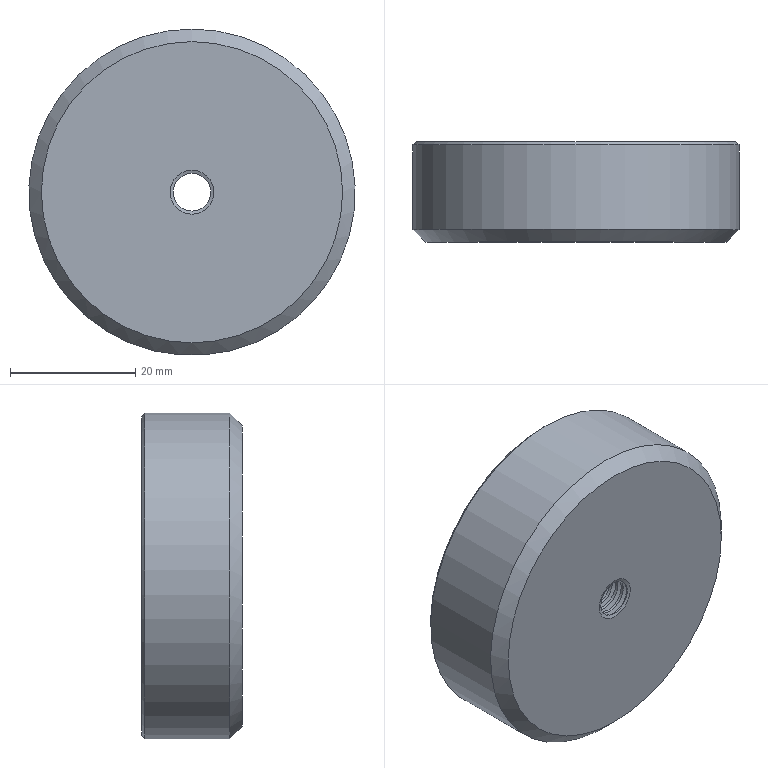Part | STEP file | PN_0003_default | 1 solid | 63 faces | box 52 x 16 x 52 mm | volume 16645 mm3 | cone 30 | cylinder 19 | torus 8 | plane 6 | commonest cylinder face diameters 6 x14 23 x1 33 x1 37 x1 48 x1 52 x1